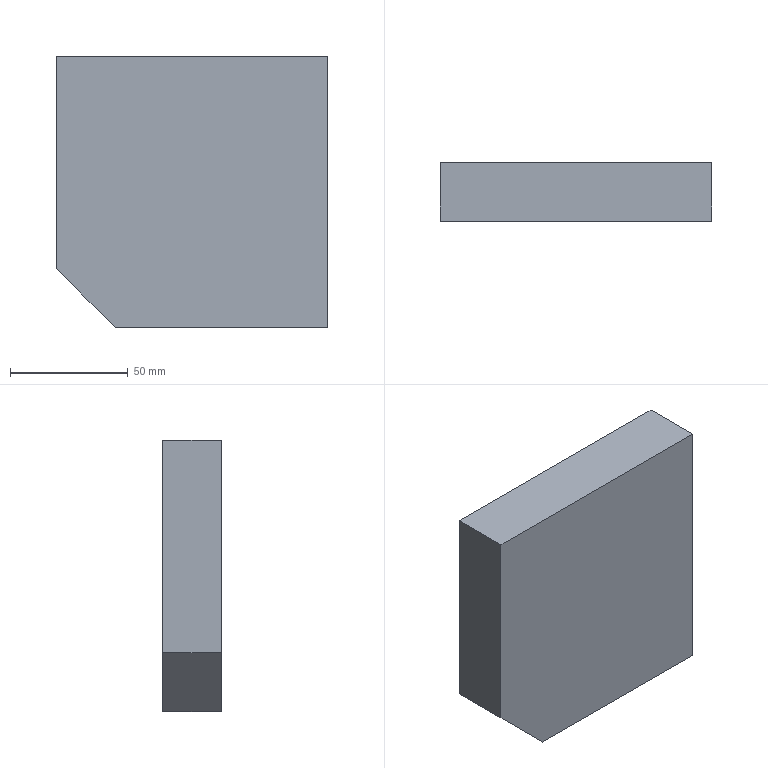Part | SolidWorks | features Extrusion 1 | 1 solid | 7 faces | box 115 x 25 x 115 mm | volume 322812 mm3 | plane 7
STEP:
#1=CARTESIAN_POINT('',(0.,0.,0.));
#2=VERTEX_POINT('',#1);
#3=CARTESIAN_POINT('',(0.,0.,-115.));
#4=VERTEX_POINT('',#3);
#5=CARTESIAN_POINT('',(0.,0.,0.));
#6=DIRECTION('',(0.,0.,-1.));
#7=VECTOR('',#6,1000.);
#8=LINE('',#5,#7);
#9=EDGE_CURVE('',#2,#4,#8,.T.);
#10=ORIENTED_EDGE('',*,*,#9,.T.);
#11=CARTESIAN_POINT('',(0.,25.,-115.));
#12=VERTEX_POINT('',#11);
#13=CARTESIAN_POINT('',(0.,25.,-115.));
#14=DIRECTION('',(0.,-1.,0.));
#15=VECTOR('',#14,1000.);
#16=LINE('',#13,#15);
#17=EDGE_CURVE('',#12,#4,#16,.T.);
#18=ORIENTED_EDGE('',*,*,#17,.F.);
#19=CARTESIAN_POINT('',(0.,25.,0.));
#20=VERTEX_POINT('',#19);
#21=CARTESIAN_POINT('',(0.,25.,0.));
#22=DIRECTION('',(0.,0.,-1.));
#23=VECTOR('',#22,1000.);
#24=LINE('',#21,#23);
#25=EDGE_CURVE('',#20,#12,#24,.T.);
#26=ORIENTED_EDGE('',*,*,#25,.F.);
#27=CARTESIAN_POINT('',(0.,25.,0.));
#28=DIRECTION('',(0.,-1.,0.));
#29=VECTOR('',#28,1000.);
#30=LINE('',#27,#29);
#31=EDGE_CURVE('',#20,#2,#30,.T.);
#32=ORIENTED_EDGE('',*,*,#31,.T.);
#33=EDGE_LOOP('',(#10,#18,#26,#32));
#34=FACE_OUTER_BOUND('',#33,.T.);
#35=CARTESIAN_POINT('',(0.,25.,0.));
#36=DIRECTION('',(-1.,0.,0.));
#37=DIRECTION('',(0.,0.,1.));
#38=AXIS2_PLACEMENT_3D('',#35,#36,#37);
#39=PLANE('',#38);
#40=ADVANCED_FACE('',(#34),#39,.F.);
#41=CARTESIAN_POINT('',(-90.,0.,-115.));
#42=VERTEX_POINT('',#41);
#43=CARTESIAN_POINT('',(0.,0.,-115.));
#44=DIRECTION('',(-1.,0.,0.));
#45=VECTOR('',#44,1000.);
#46=LINE('',#43,#45);
#47=EDGE_CURVE('',#4,#42,#46,.T.);
#48=ORIENTED_EDGE('',*,*,#47,.T.);
#49=CARTESIAN_POINT('',(-90.,25.,-115.));
#50=VERTEX_POINT('',#49);
#51=CARTESIAN_POINT('',(-90.,25.,-115.));
#52=DIRECTION('',(0.,-1.,0.));
#53=VECTOR('',#52,1000.);
#54=LINE('',#51,#53);
#55=EDGE_CURVE('',#50,#42,#54,.T.);
#56=ORIENTED_EDGE('',*,*,#55,.F.);
#57=CARTESIAN_POINT('',(0.,25.,-115.));
#58=DIRECTION('',(-1.,0.,0.));
#59=VECTOR('',#58,1000.);
#60=LINE('',#57,#59);
#61=EDGE_CURVE('',#12,#50,#60,.T.);
#62=ORIENTED_EDGE('',*,*,#61,.F.);
#63=ORIENTED_EDGE('',*,*,#17,.T.);
#64=EDGE_LOOP('',(#48,#56,#62,#63));
#65=FACE_OUTER_BOUND('',#64,.T.);
#66=CARTESIAN_POINT('',(0.,25.,-115.));
#67=DIRECTION('',(0.,0.,1.));
#68=DIRECTION('',(1.,0.,0.));
#69=AXIS2_PLACEMENT_3D('',#66,#67,#68);
#70=PLANE('',#69);
#71=ADVANCED_FACE('',(#65),#70,.F.);
#72=CARTESIAN_POINT('',(-115.,0.,-90.));
#73=VERTEX_POINT('',#72);
#74=CARTESIAN_POINT('',(-115.,0.,-90.));
#75=DIRECTION('',(-0.7071,0.,0.7071));
#76=VECTOR('',#75,1000.);
#77=LINE('',#74,#76);
#78=EDGE_CURVE('',#42,#73,#77,.T.);
#79=ORIENTED_EDGE('',*,*,#78,.T.);
#80=CARTESIAN_POINT('',(-115.,25.,-90.));
#81=VERTEX_POINT('',#80);
#82=CARTESIAN_POINT('',(-115.,25.,-90.));
#83=DIRECTION('',(0.,-1.,0.));
#84=VECTOR('',#83,1000.);
#85=LINE('',#82,#84);
#86=EDGE_CURVE('',#81,#73,#85,.T.);
#87=ORIENTED_EDGE('',*,*,#86,.F.);
#88=CARTESIAN_POINT('',(-115.,25.,-90.));
#89=DIRECTION('',(-0.7071,0.,0.7071));
#90=VECTOR('',#89,1000.);
#91=LINE('',#88,#90);
#92=EDGE_CURVE('',#50,#81,#91,.T.);
#93=ORIENTED_EDGE('',*,*,#92,.F.);
#94=ORIENTED_EDGE('',*,*,#55,.T.);
#95=EDGE_LOOP('',(#79,#87,#93,#94));
#96=FACE_OUTER_BOUND('',#95,.T.);
#97=CARTESIAN_POINT('',(-115.,25.,-90.));
#98=DIRECTION('',(0.7071,0.,0.7071));
#99=DIRECTION('',(0.7071,0.,-0.7071));
#100=AXIS2_PLACEMENT_3D('',#97,#98,#99);
#101=PLANE('',#100);
#102=ADVANCED_FACE('',(#96),#101,.F.);
#103=CARTESIAN_POINT('',(-115.,0.,0.));
#104=VERTEX_POINT('',#103);
#105=CARTESIAN_POINT('',(-115.,0.,0.));
#106=DIRECTION('',(0.,0.,1.));
#107=VECTOR('',#106,1000.);
#108=LINE('',#105,#107);
#109=EDGE_CURVE('',#73,#104,#108,.T.);
#110=ORIENTED_EDGE('',*,*,#109,.T.);
#111=CARTESIAN_POINT('',(-115.,25.,0.));
#112=VERTEX_POINT('',#111);
#113=CARTESIAN_POINT('',(-115.,25.,0.));
#114=DIRECTION('',(0.,-1.,0.));
#115=VECTOR('',#114,1000.);
#116=LINE('',#113,#115);
#117=EDGE_CURVE('',#112,#104,#116,.T.);
#118=ORIENTED_EDGE('',*,*,#117,.F.);
#119=CARTESIAN_POINT('',(-115.,25.,0.));
#120=DIRECTION('',(0.,0.,1.));
#121=VECTOR('',#120,1000.);
#122=LINE('',#119,#121);
#123=EDGE_CURVE('',#81,#112,#122,.T.);
#124=ORIENTED_EDGE('',*,*,#123,.F.);
#125=ORIENTED_EDGE('',*,*,#86,.T.);
#126=EDGE_LOOP('',(#110,#118,#124,#125));
#127=FACE_OUTER_BOUND('',#126,.T.);
#128=CARTESIAN_POINT('',(-115.,25.,0.));
#129=DIRECTION('',(1.,0.,0.));
#130=DIRECTION('',(0.,0.,-1.));
#131=AXIS2_PLACEMENT_3D('',#128,#129,#130);
#132=PLANE('',#131);
#133=ADVANCED_FACE('',(#127),#132,.F.);
#134=CARTESIAN_POINT('',(0.,0.,0.));
#135=DIRECTION('',(1.,0.,0.));
#136=VECTOR('',#135,1000.);
#137=LINE('',#134,#136);
#138=EDGE_CURVE('',#104,#2,#137,.T.);
#139=ORIENTED_EDGE('',*,*,#138,.T.);
#140=ORIENTED_EDGE('',*,*,#31,.F.);
#141=CARTESIAN_POINT('',(0.,25.,0.));
#142=DIRECTION('',(1.,0.,0.));
#143=VECTOR('',#142,1000.);
#144=LINE('',#141,#143);
#145=EDGE_CURVE('',#112,#20,#144,.T.);
#146=ORIENTED_EDGE('',*,*,#145,.F.);
#147=ORIENTED_EDGE('',*,*,#117,.T.);
#148=EDGE_LOOP('',(#139,#140,#146,#147));
#149=FACE_OUTER_BOUND('',#148,.T.);
#150=CARTESIAN_POINT('',(0.,25.,0.));
#151=DIRECTION('',(0.,0.,-1.));
#152=DIRECTION('',(-1.,0.,0.));
#153=AXIS2_PLACEMENT_3D('',#150,#151,#152);
#154=PLANE('',#153);
#155=ADVANCED_FACE('',(#149),#154,.F.);
#156=ORIENTED_EDGE('',*,*,#25,.T.);
#157=ORIENTED_EDGE('',*,*,#61,.T.);
#158=ORIENTED_EDGE('',*,*,#92,.T.);
#159=ORIENTED_EDGE('',*,*,#123,.T.);
#160=ORIENTED_EDGE('',*,*,#145,.T.);
#161=EDGE_LOOP('',(#156,#157,#158,#159,#160));
#162=FACE_OUTER_BOUND('',#161,.T.);
#163=CARTESIAN_POINT('',(0.,25.,0.));
#164=DIRECTION('',(0.,1.,0.));
#165=DIRECTION('',(0.,0.,1.));
#166=AXIS2_PLACEMENT_3D('',#163,#164,#165);
#167=PLANE('',#166);
#168=ADVANCED_FACE('',(#162),#167,.T.);
#169=ORIENTED_EDGE('',*,*,#9,.F.);
#170=ORIENTED_EDGE('',*,*,#138,.F.);
#171=ORIENTED_EDGE('',*,*,#109,.F.);
#172=ORIENTED_EDGE('',*,*,#78,.F.);
#173=ORIENTED_EDGE('',*,*,#47,.F.);
#174=EDGE_LOOP('',(#169,#170,#171,#172,#173));
#175=FACE_OUTER_BOUND('',#174,.T.);
#176=CARTESIAN_POINT('',(0.,0.,0.));
#177=DIRECTION('',(0.,1.,0.));
#178=DIRECTION('',(0.,0.,1.));
#179=AXIS2_PLACEMENT_3D('',#176,#177,#178);
#180=PLANE('',#179);
#181=ADVANCED_FACE('',(#175),#180,.F.);
#182=CLOSED_SHELL('',(#40,#71,#102,#133,#155,#168,#181));
#183=MANIFOLD_SOLID_BREP('',#182);
#184=CARTESIAN_POINT('',(0.,0.,0.));
#185=DIRECTION('',(0.,0.,1.));
#186=DIRECTION('',(1.,0.,0.));
#187=AXIS2_PLACEMENT_3D('',#184,#185,#186);
#188=(LENGTH_UNIT()NAMED_UNIT(*)SI_UNIT(.MILLI.,.METRE.));
#189=UNCERTAINTY_MEASURE_WITH_UNIT(LENGTH_MEASURE(0.00001),#188,'','');
#190=(NAMED_UNIT(*)PLANE_ANGLE_UNIT()SI_UNIT($,.RADIAN.));
#191=(NAMED_UNIT(*)SI_UNIT($,.STERADIAN.)SOLID_ANGLE_UNIT());
#192=(GEOMETRIC_REPRESENTATION_CONTEXT(3)GLOBAL_UNCERTAINTY_ASSIGNED_CONTEXT((#189))GLOBAL_UNIT_ASSIGNED_CONTEXT((#188,#190,#191))REPRESENTATION_CONTEXT('',''));
#193=ADVANCED_BREP_SHAPE_REPRESENTATION('',(#183,#187),#192);